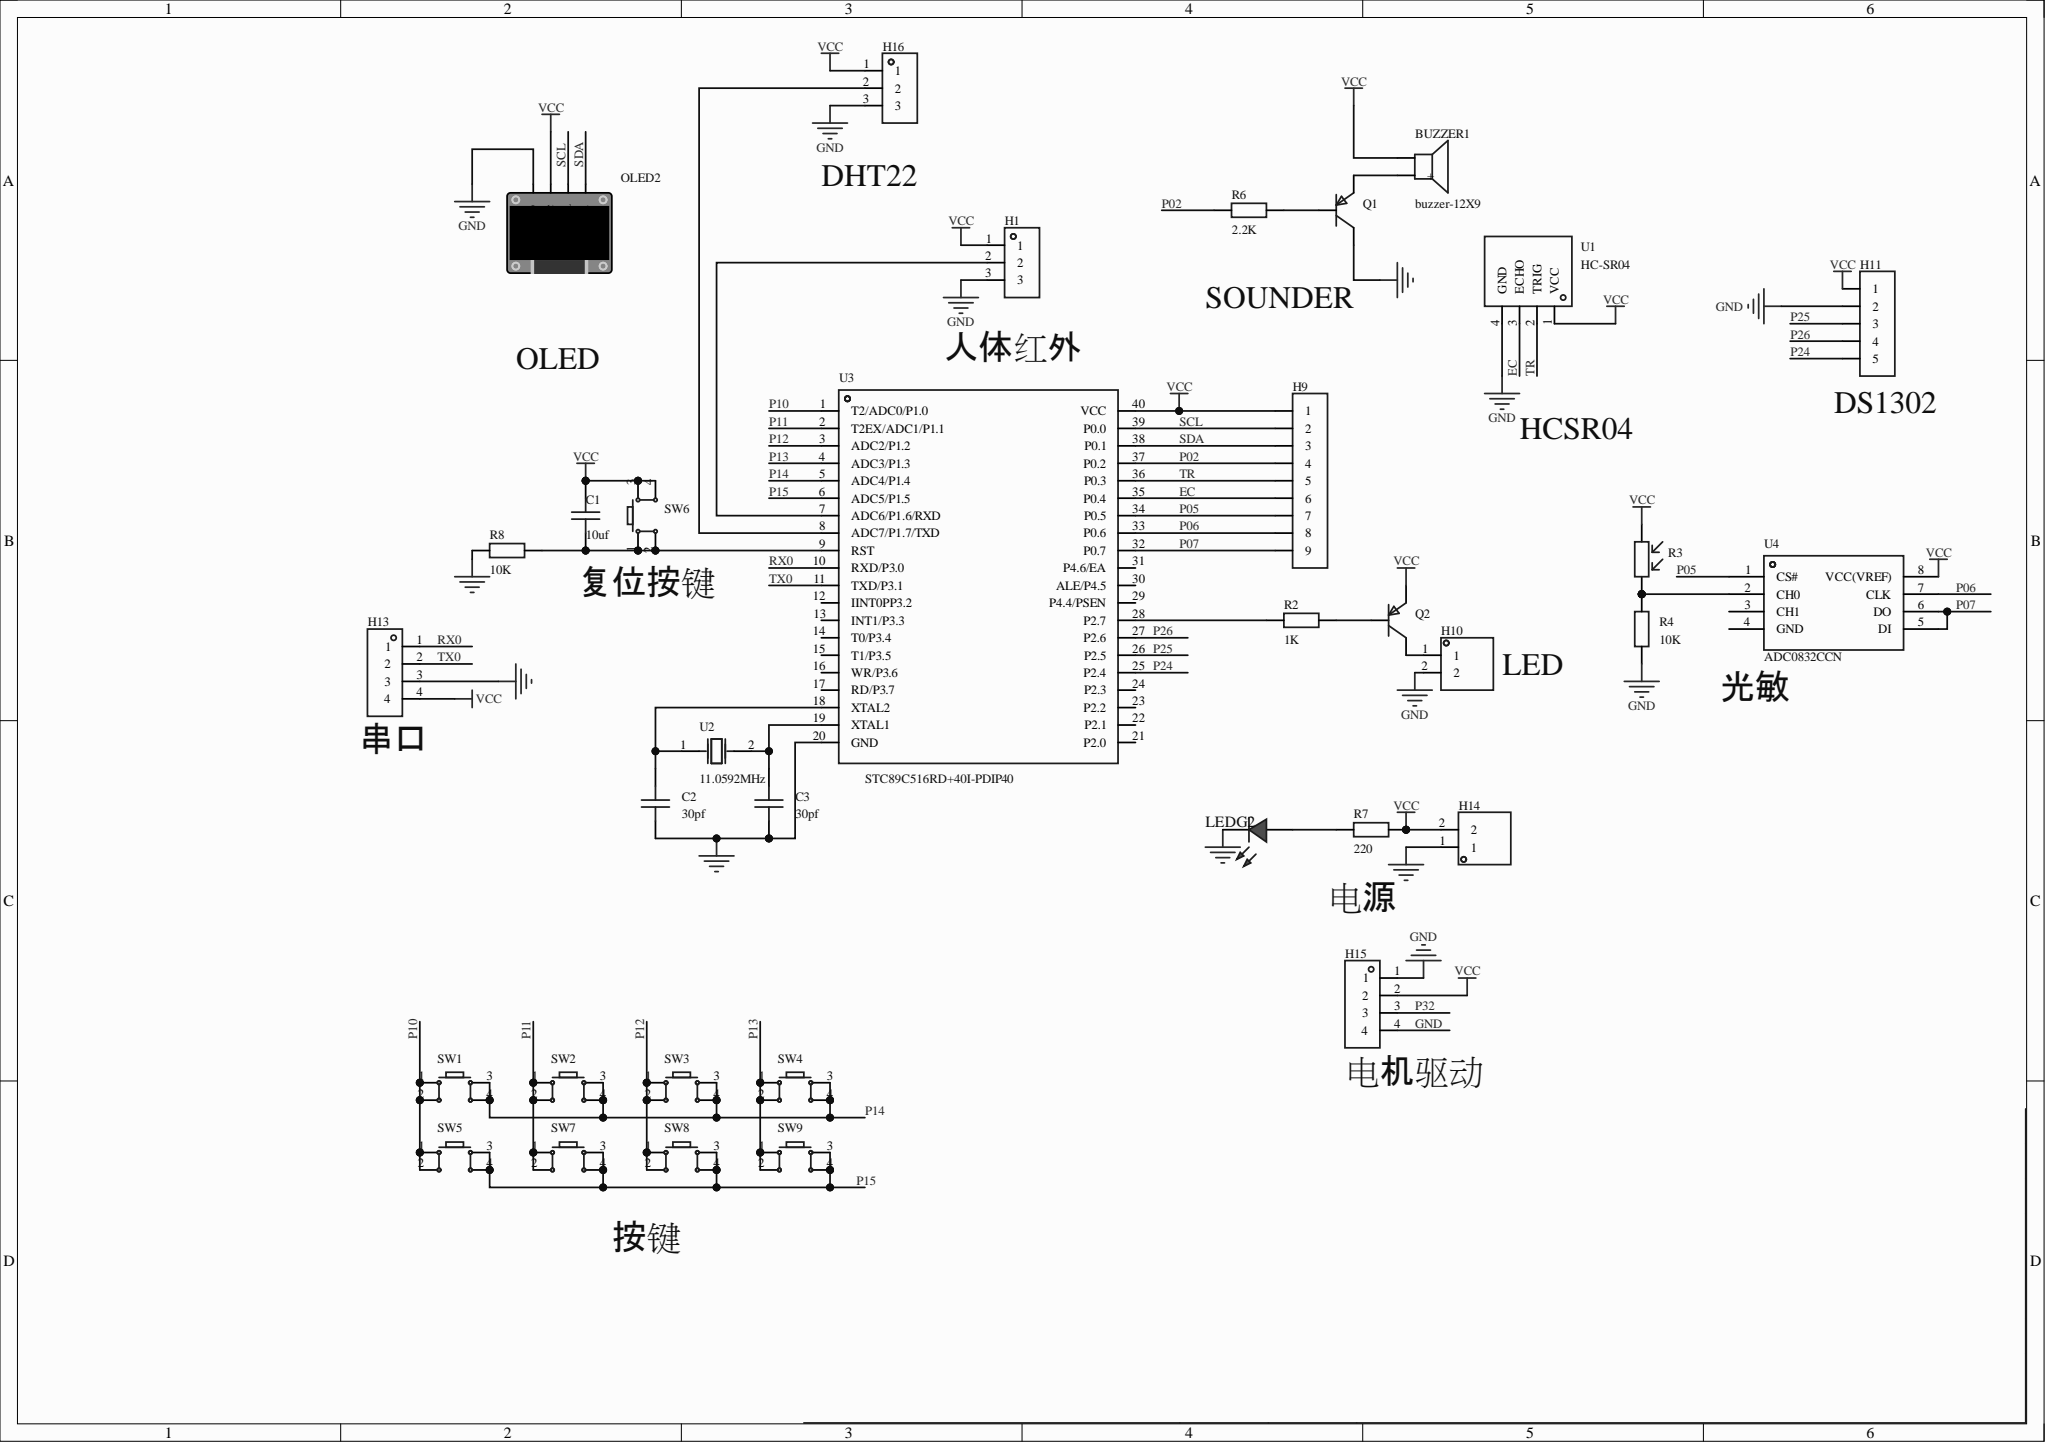Circuit board | Altium Designer | 35 parts | 33 nets
Bill of materials:
Comment,Description,Designator,Footprint,LibRef,Quantity
"buzzer-12X9","","BUZZER1","BUZ-TH_BD12.0-P7.60-D0.6-FD","buzzer-12X9","1"
"10uf","","C1","C0805","CAP_0805","1"
"30pf","","C2, C3","C0805","CAP_0805","2"
"","","H1, H16","HDR-TH_3P-P2.54-V-F","HDR-F_2.54_1x3P","2"
"","","H9","HDR-TH_9P-P2.54-V-F-1","HDR-F_2.54_1x9P","1"
"","","H10, H14","HDR-TH_2P-P2.54-V-M-1","HDR-M_2.54_1x2P","2"
"","","H11","HDR-TH_5P-P2.54-V-F","HDR-F_2.54_1x5P","1"
"","","H13","HDR-TH_4P-P2.54-V-M","HDR-M_2.54_1x4P","1"
"","","H15","HDR-TH_4P-P2.54-V-F","HDR-F_2.54_1x4P","1"
"","","LEDG2","LED_0805","LED_0805-R","1"
"","","OLED2","0.96OLED_4P","0.96OLED模块_4P","1"
"2N3906S-RTK/PS","","Q1","SOT-23-3_L2.9-W1.3-P1.90-LS2.4-TR","2N3906S-RTK/PS","1"
"","","Q2","S8550P_SOT","S8550_SOT_PNP","1"
"1K","","R2","R0805","Res_0805","1"
"GL5549(80-100)","","R3","RES-TH_L5.1-W4.3-P3.40-D0.5","GL5549(80-100)","1"
"10K","","R4, R8","R0805","Res_0805","2"
"2.2K","","R6","R0805","Res_0805","1"
"220","","R7","R0805","Res_0805","1"
"","","SW1, SW2, SW3, SW4, SW5, SW6, SW7, SW8, SW9","SW-TH_4P-L6.0-W6.0-P4.50-LS6.5","Key_TH_6x6x6","9"
"HC-SR04","","U1","TH_HC-SR04V","HC-SR04","1"
"11.059MHz","频率:12MHz;常温频差:±30ppm;外接负载电容:-;频率稳定度(全温):±50ppm;","U2","HC-49US_L11.0-W4.6-P4.88","ECS-120-S-4","1"
"STC89C516RD+40I-PDIP40","CPU内核:51系列;程序存储容量:61KB;RAM总容量:1.25KB;GPIO端口数量:35;工作电压范围:3.5V~5.5V;CPU最大主频:-;程序存储器类型:FLASH;","U3","DIP-40_L52.3-W13.9-P2.54-LS15.2-BL","STC89C516RD+40I-PDIP40","1"
"ADC0832CCN","","U4","DIP-8_L9.7-W6.4-P2.54-LS7.6-BL","ADC0832CCN","1"
Netlist (Protel format):
[
BUZZER1
BUZ-TH_BD12.0-P7.60-D0.6-FD
buzzer-12X9



]
[
C1
C0805
10uf



]
[
C2
C0805
30pf



]
[
C3
C0805
30pf



]
[
H1
HDR-TH_3P-P2.54-V-F




]
[
H9
HDR-TH_9P-P2.54-V-F-1




]
[
H10
HDR-TH_2P-P2.54-V-M-1




]
[
H11
HDR-TH_5P-P2.54-V-F




]
[
H13
HDR-TH_4P-P2.54-V-M




]
[
H14
HDR-TH_2P-P2.54-V-M-1




]
[
H15
HDR-TH_4P-P2.54-V-F




]
[
H16
HDR-TH_3P-P2.54-V-F




]
[
LEDG2
LED_0805




]
[
OLED2
0.96OLED_4P




]
[
Q1
SOT-23-3_L2.9-W1.3-P1.90-LS2.4-TR
2N3906S-RTK/PS



]
[
Q2
S8550P_SOT




]
[
R2
R0805
1K



]
[
R3
RES-TH_L5.1-W4.3-P3.40-D0.5
GL5549(80-100)



]
[
R4
R0805
10K



]
[
R6
R0805
2.2K



]
[
R7
R0805
220



]
[
R8
R0805
10K



]
[
SW1
SW-TH_4P-L6.0-W6.0-P4.50-LS6.5




]
[
SW2
SW-TH_4P-L6.0-W6.0-P4.50-LS6.5




]
[
SW3
SW-TH_4P-L6.0-W6.0-P4.50-LS6.5




]
[
SW4
SW-TH_4P-L6.0-W6.0-P4.50-LS6.5




]
[
SW5
SW-TH_4P-L6.0-W6.0-P4.50-LS6.5




]
[
SW6
SW-TH_4P-L6.0-W6.0-P4.50-LS6.5




]
[
SW7
SW-TH_4P-L6.0-W6.0-P4.50-LS6.5




]
[
SW8
SW-TH_4P-L6.0-W6.0-P4.50-LS6.5




]
[
SW9
SW-TH_4P-L6.0-W6.0-P4.50-LS6.5




]
[
U1
TH_HC-SR04V
HC-SR04



]
[
U2
HC-49US_L11.0-W4.6-P4.88
11.0592MHz



]
[
U3
DIP-40_L52.3-W13.9-P2.54-LS15.2-BL
STC89C516RD+40I-PDIP40



]
[
U4
DIP-8_L9.7-W6.4-P2.54-LS7.6-BL
ADC0832CCN



]
(
VCC
BUZZER1-2
C1-2
H1-1
H9-1
H11-1
H13-4
H14-2
H15-2
H16-1
OLED2-2
Q2-2
R3-1
R7-2
SW6-3
SW6-4
U1-1
U3-40
U4-8
)
(
TX0
H13-2
U3-11
)
(
TR
H9-5
U1-2
U3-36
)
(
SDA
H9-3
OLED2-4
U3-38
)
(
SCL
H9-2
OLED2-3
U3-39
)
(
RX0
H13-1
U3-10
)
(
P26
H11-4
U3-27
)
(
P25
H11-3
U3-26
)
(
P24
H11-5
U3-25
)
(
P15
SW5-3
SW5-4
SW7-3
SW7-4
SW8-3
SW8-4
SW9-3
SW9-4
U3-6
)
(
P14
SW1-3
SW1-4
SW2-3
SW2-4
SW3-3
SW3-4
SW4-3
SW4-4
U3-5
)
(
P13
SW4-1
SW4-2
SW9-1
SW9-2
U3-4
)
(
P12
SW3-1
SW3-2
SW8-1
SW8-2
U3-3
)
(
P11
SW2-1
SW2-2
SW7-1
SW7-2
U3-2
)
(
P10
SW1-1
SW1-2
SW5-1
SW5-2
U3-1
)
(
P07
H9-9
U3-32
U4-5
U4-6
)
(
P06
H9-8
U3-33
U4-7
)
(
P05
H9-7
U3-34
U4-1
)
(
P02
H9-4
R6-1
U3-37
)
(
NetR3_2
R3-2
R4-2
U4-2
)
(
NetR2_1
R2-1
U3-28
)
(
NetQ2_1
Q2-1
R2-2
)
(
NetQ1_2
Q1-2
R6-2
)
(
NetLEDG2_2
LEDG2-2
R7-1
)
(
NetH16_2
H16-2
U3-8
)
(
NetH10_1
H10-1
Q2-3
)
(
NetH1_2
H1-2
U3-7
)
(
NetC3_2
C3-2
U2-2
U3-19
)
(
NetC2_2
C2-2
U2-1
U3-18
)
(
NetC1_1
C1-1
R8-1
SW6-1
SW6-2
U3-9
)
(
NetBUZZER1_1
BUZZER1-1
Q1-1
)
(
GND
C2-1
C3-1
H1-3
H10-2
H11-2
H13-3
H14-1
H15-1
H15-4
H16-3
LEDG2-1
OLED2-1
Q1-3
R4-1
R8-2
U1-4
U3-20
)
(
EC
H9-6
U1-3
U3-35
)